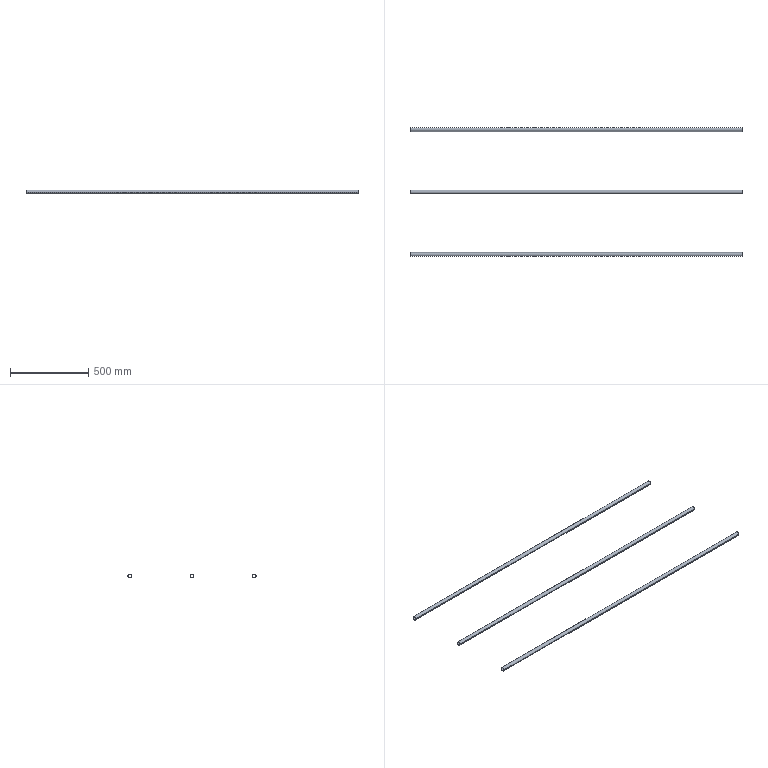Part | STEP file | Powder bin guardrail rail 5_Default<As Machined> | 3 solids | 18 faces | box 2128 x 825 x 25 mm | volume 706805 mm3 | cylinder 12 | plane 6 | commonest cylinder face diameters 22 x6 25 x6
STEP:
#1=CARTESIAN_POINT('',(0.,0.,0.));
#2=DIRECTION('',(0.,0.,1.));
#3=DIRECTION('',(1.,0.,0.));
#4=AXIS2_PLACEMENT_3D('',#1,#2,#3);
#5=CARTESIAN_POINT('',(1063.75,812.5,0.));
#6=VERTEX_POINT('',#5);
#7=CARTESIAN_POINT('',(1063.75,787.5,0.));
#8=VERTEX_POINT('',#7);
#9=CARTESIAN_POINT('',(1063.75,800.,0.));
#10=DIRECTION('',(1.,0.,0.));
#11=DIRECTION('',(0.,1.,0.));
#12=AXIS2_PLACEMENT_3D('',#9,#10,#11);
#13=CIRCLE('',#12,12.5);
#14=CARTESIAN_POINT('',(1063.75,800.,0.));
#15=DIRECTION('',(-1.,0.,0.));
#16=DIRECTION('',(0.,-1.,0.));
#17=AXIS2_PLACEMENT_3D('',#14,#15,#16);
#18=CYLINDRICAL_SURFACE('',#17,12.5);
#19=CARTESIAN_POINT('',(3.142,0.));
#20=DIRECTION('',(-1.,0.));
#21=VECTOR('',#20,1.);
#22=LINE('',#19,#21);
#23=(GEOMETRIC_REPRESENTATION_CONTEXT(2)PARAMETRIC_REPRESENTATION_CONTEXT()REPRESENTATION_CONTEXT('',''));
#24=DEFINITIONAL_REPRESENTATION('',(#22),#23);
#25=PCURVE('',#18,#24);
#26=CARTESIAN_POINT('',(1063.75,800.,0.));
#27=DIRECTION('',(1.,0.,0.));
#28=DIRECTION('',(0.,1.,0.));
#29=AXIS2_PLACEMENT_3D('',#26,#27,#28);
#30=PLANE('',#29);
#31=CARTESIAN_POINT('',(0.,0.));
#32=DIRECTION('',(1.,0.));
#33=AXIS2_PLACEMENT_2D('',#31,#32);
#34=CIRCLE('',#33,12.5);
#35=(GEOMETRIC_REPRESENTATION_CONTEXT(2)PARAMETRIC_REPRESENTATION_CONTEXT()REPRESENTATION_CONTEXT('',''));
#36=DEFINITIONAL_REPRESENTATION('',(#34),#35);
#37=PCURVE('',#30,#36);
#38=SURFACE_CURVE('',#13,(#25,#37),.PCURVE_S1.);
#39=EDGE_CURVE('',#6,#8,#38,.T.);
#40=ORIENTED_EDGE('',*,*,#39,.F.);
#41=CARTESIAN_POINT('',(-1063.75,812.5,0.));
#42=VERTEX_POINT('',#41);
#43=CARTESIAN_POINT('',(1063.75,812.5,0.));
#44=DIRECTION('',(-1.,0.,0.));
#45=VECTOR('',#44,1.);
#46=LINE('',#43,#45);
#47=CARTESIAN_POINT('',(3.142,0.));
#48=DIRECTION('',(0.,1.));
#49=VECTOR('',#48,1.);
#50=LINE('',#47,#49);
#51=(GEOMETRIC_REPRESENTATION_CONTEXT(2)PARAMETRIC_REPRESENTATION_CONTEXT()REPRESENTATION_CONTEXT('',''));
#52=DEFINITIONAL_REPRESENTATION('',(#50),#51);
#53=PCURVE('',#18,#52);
#54=CARTESIAN_POINT('',(1063.75,800.,0.));
#55=DIRECTION('',(-1.,0.,0.));
#56=DIRECTION('',(0.,-1.,0.));
#57=AXIS2_PLACEMENT_3D('',#54,#55,#56);
#58=CYLINDRICAL_SURFACE('',#57,12.5);
#59=CARTESIAN_POINT('',(3.142,0.));
#60=DIRECTION('',(0.,1.));
#61=VECTOR('',#60,1.);
#62=LINE('',#59,#61);
#63=(GEOMETRIC_REPRESENTATION_CONTEXT(2)PARAMETRIC_REPRESENTATION_CONTEXT()REPRESENTATION_CONTEXT('',''));
#64=DEFINITIONAL_REPRESENTATION('',(#62),#63);
#65=PCURVE('',#58,#64);
#66=SURFACE_CURVE('',#46,(#53,#65),.PCURVE_S1.);
#67=EDGE_CURVE('',#6,#42,#66,.T.);
#68=ORIENTED_EDGE('',*,*,#67,.T.);
#69=CARTESIAN_POINT('',(-1063.75,787.5,0.));
#70=VERTEX_POINT('',#69);
#71=CARTESIAN_POINT('',(-1063.75,800.,0.));
#72=DIRECTION('',(1.,0.,0.));
#73=DIRECTION('',(0.,1.,0.));
#74=AXIS2_PLACEMENT_3D('',#71,#72,#73);
#75=CIRCLE('',#74,12.5);
#76=CARTESIAN_POINT('',(3.142,2127.5));
#77=DIRECTION('',(-1.,0.));
#78=VECTOR('',#77,1.);
#79=LINE('',#76,#78);
#80=(GEOMETRIC_REPRESENTATION_CONTEXT(2)PARAMETRIC_REPRESENTATION_CONTEXT()REPRESENTATION_CONTEXT('',''));
#81=DEFINITIONAL_REPRESENTATION('',(#79),#80);
#82=PCURVE('',#18,#81);
#83=CARTESIAN_POINT('',(-1063.75,800.,0.));
#84=DIRECTION('',(1.,0.,0.));
#85=DIRECTION('',(0.,1.,0.));
#86=AXIS2_PLACEMENT_3D('',#83,#84,#85);
#87=PLANE('',#86);
#88=CARTESIAN_POINT('',(0.,0.));
#89=DIRECTION('',(1.,0.));
#90=AXIS2_PLACEMENT_2D('',#88,#89);
#91=CIRCLE('',#90,12.5);
#92=(GEOMETRIC_REPRESENTATION_CONTEXT(2)PARAMETRIC_REPRESENTATION_CONTEXT()REPRESENTATION_CONTEXT('',''));
#93=DEFINITIONAL_REPRESENTATION('',(#91),#92);
#94=PCURVE('',#87,#93);
#95=SURFACE_CURVE('',#75,(#82,#94),.PCURVE_S1.);
#96=EDGE_CURVE('',#42,#70,#95,.T.);
#97=ORIENTED_EDGE('',*,*,#96,.T.);
#98=CARTESIAN_POINT('',(1063.75,787.5,0.));
#99=DIRECTION('',(-1.,0.,0.));
#100=VECTOR('',#99,1.);
#101=LINE('',#98,#100);
#102=CARTESIAN_POINT('',(0.,0.));
#103=DIRECTION('',(0.,1.));
#104=VECTOR('',#103,1.);
#105=LINE('',#102,#104);
#106=(GEOMETRIC_REPRESENTATION_CONTEXT(2)PARAMETRIC_REPRESENTATION_CONTEXT()REPRESENTATION_CONTEXT('',''));
#107=DEFINITIONAL_REPRESENTATION('',(#105),#106);
#108=PCURVE('',#18,#107);
#109=CARTESIAN_POINT('',(6.283,0.));
#110=DIRECTION('',(0.,1.));
#111=VECTOR('',#110,1.);
#112=LINE('',#109,#111);
#113=(GEOMETRIC_REPRESENTATION_CONTEXT(2)PARAMETRIC_REPRESENTATION_CONTEXT()REPRESENTATION_CONTEXT('',''));
#114=DEFINITIONAL_REPRESENTATION('',(#112),#113);
#115=PCURVE('',#58,#114);
#116=SURFACE_CURVE('',#101,(#108,#115),.PCURVE_S1.);
#117=EDGE_CURVE('',#8,#70,#116,.T.);
#118=ORIENTED_EDGE('',*,*,#117,.F.);
#119=EDGE_LOOP('',(#40,#68,#97,#118));
#120=FACE_BOUND('',#119,.T.);
#121=ADVANCED_FACE('',(#120),#18,.T.);
#122=CARTESIAN_POINT('',(1063.75,789.,0.));
#123=VERTEX_POINT('',#122);
#124=CARTESIAN_POINT('',(-1063.75,789.,0.));
#125=VERTEX_POINT('',#124);
#126=CARTESIAN_POINT('',(1063.75,789.,0.));
#127=DIRECTION('',(-1.,0.,0.));
#128=VECTOR('',#127,1.);
#129=LINE('',#126,#128);
#130=CARTESIAN_POINT('',(1063.75,800.,0.));
#131=DIRECTION('',(-1.,0.,0.));
#132=DIRECTION('',(0.,-1.,0.));
#133=AXIS2_PLACEMENT_3D('',#130,#131,#132);
#134=CYLINDRICAL_SURFACE('',#133,11.);
#135=CARTESIAN_POINT('',(6.283,0.));
#136=DIRECTION('',(0.,1.));
#137=VECTOR('',#136,1.);
#138=LINE('',#135,#137);
#139=(GEOMETRIC_REPRESENTATION_CONTEXT(2)PARAMETRIC_REPRESENTATION_CONTEXT()REPRESENTATION_CONTEXT('',''));
#140=DEFINITIONAL_REPRESENTATION('',(#138),#139);
#141=PCURVE('',#134,#140);
#142=CARTESIAN_POINT('',(1063.75,800.,0.));
#143=DIRECTION('',(-1.,0.,0.));
#144=DIRECTION('',(0.,-1.,0.));
#145=AXIS2_PLACEMENT_3D('',#142,#143,#144);
#146=CYLINDRICAL_SURFACE('',#145,11.);
#147=CARTESIAN_POINT('',(0.,0.));
#148=DIRECTION('',(0.,1.));
#149=VECTOR('',#148,1.);
#150=LINE('',#147,#149);
#151=(GEOMETRIC_REPRESENTATION_CONTEXT(2)PARAMETRIC_REPRESENTATION_CONTEXT()REPRESENTATION_CONTEXT('',''));
#152=DEFINITIONAL_REPRESENTATION('',(#150),#151);
#153=PCURVE('',#146,#152);
#154=SURFACE_CURVE('',#129,(#141,#153),.PCURVE_S1.);
#155=EDGE_CURVE('',#123,#125,#154,.T.);
#156=ORIENTED_EDGE('',*,*,#155,.T.);
#157=CARTESIAN_POINT('',(-1063.75,811.,0.));
#158=VERTEX_POINT('',#157);
#159=CARTESIAN_POINT('',(-1063.75,800.,0.));
#160=DIRECTION('',(1.,0.,0.));
#161=DIRECTION('',(0.,1.,0.));
#162=AXIS2_PLACEMENT_3D('',#159,#160,#161);
#163=CIRCLE('',#162,11.);
#164=CARTESIAN_POINT('',(9.425,2127.5));
#165=DIRECTION('',(-1.,0.));
#166=VECTOR('',#165,1.);
#167=LINE('',#164,#166);
#168=(GEOMETRIC_REPRESENTATION_CONTEXT(2)PARAMETRIC_REPRESENTATION_CONTEXT()REPRESENTATION_CONTEXT('',''));
#169=DEFINITIONAL_REPRESENTATION('',(#167),#168);
#170=PCURVE('',#134,#169);
#171=CARTESIAN_POINT('',(0.,0.));
#172=DIRECTION('',(1.,0.));
#173=AXIS2_PLACEMENT_2D('',#171,#172);
#174=CIRCLE('',#173,11.);
#175=(GEOMETRIC_REPRESENTATION_CONTEXT(2)PARAMETRIC_REPRESENTATION_CONTEXT()REPRESENTATION_CONTEXT('',''));
#176=DEFINITIONAL_REPRESENTATION('',(#174),#175);
#177=PCURVE('',#87,#176);
#178=SURFACE_CURVE('',#163,(#170,#177),.PCURVE_S1.);
#179=EDGE_CURVE('',#125,#158,#178,.T.);
#180=ORIENTED_EDGE('',*,*,#179,.T.);
#181=CARTESIAN_POINT('',(1063.75,811.,0.));
#182=VERTEX_POINT('',#181);
#183=CARTESIAN_POINT('',(1063.75,811.,0.));
#184=DIRECTION('',(-1.,0.,0.));
#185=VECTOR('',#184,1.);
#186=LINE('',#183,#185);
#187=CARTESIAN_POINT('',(3.142,0.));
#188=DIRECTION('',(0.,1.));
#189=VECTOR('',#188,1.);
#190=LINE('',#187,#189);
#191=(GEOMETRIC_REPRESENTATION_CONTEXT(2)PARAMETRIC_REPRESENTATION_CONTEXT()REPRESENTATION_CONTEXT('',''));
#192=DEFINITIONAL_REPRESENTATION('',(#190),#191);
#193=PCURVE('',#134,#192);
#194=CARTESIAN_POINT('',(3.142,0.));
#195=DIRECTION('',(0.,1.));
#196=VECTOR('',#195,1.);
#197=LINE('',#194,#196);
#198=(GEOMETRIC_REPRESENTATION_CONTEXT(2)PARAMETRIC_REPRESENTATION_CONTEXT()REPRESENTATION_CONTEXT('',''));
#199=DEFINITIONAL_REPRESENTATION('',(#197),#198);
#200=PCURVE('',#146,#199);
#201=SURFACE_CURVE('',#186,(#193,#200),.PCURVE_S1.);
#202=EDGE_CURVE('',#182,#158,#201,.T.);
#203=ORIENTED_EDGE('',*,*,#202,.F.);
#204=CARTESIAN_POINT('',(1063.75,800.,0.));
#205=DIRECTION('',(1.,0.,0.));
#206=DIRECTION('',(0.,1.,0.));
#207=AXIS2_PLACEMENT_3D('',#204,#205,#206);
#208=CIRCLE('',#207,11.);
#209=CARTESIAN_POINT('',(9.425,0.));
#210=DIRECTION('',(-1.,0.));
#211=VECTOR('',#210,1.);
#212=LINE('',#209,#211);
#213=(GEOMETRIC_REPRESENTATION_CONTEXT(2)PARAMETRIC_REPRESENTATION_CONTEXT()REPRESENTATION_CONTEXT('',''));
#214=DEFINITIONAL_REPRESENTATION('',(#212),#213);
#215=PCURVE('',#134,#214);
#216=CARTESIAN_POINT('',(0.,0.));
#217=DIRECTION('',(1.,0.));
#218=AXIS2_PLACEMENT_2D('',#216,#217);
#219=CIRCLE('',#218,11.);
#220=(GEOMETRIC_REPRESENTATION_CONTEXT(2)PARAMETRIC_REPRESENTATION_CONTEXT()REPRESENTATION_CONTEXT('',''));
#221=DEFINITIONAL_REPRESENTATION('',(#219),#220);
#222=PCURVE('',#30,#221);
#223=SURFACE_CURVE('',#208,(#215,#222),.PCURVE_S1.);
#224=EDGE_CURVE('',#123,#182,#223,.T.);
#225=ORIENTED_EDGE('',*,*,#224,.F.);
#226=EDGE_LOOP('',(#156,#180,#203,#225));
#227=FACE_BOUND('',#226,.F.);
#228=ADVANCED_FACE('',(#227),#134,.F.);
#229=CARTESIAN_POINT('',(-1063.75,800.,0.));
#230=DIRECTION('',(1.,0.,0.));
#231=DIRECTION('',(0.,1.,0.));
#232=AXIS2_PLACEMENT_3D('',#229,#230,#231);
#233=CIRCLE('',#232,11.);
#234=CARTESIAN_POINT('',(3.142,2127.5));
#235=DIRECTION('',(-1.,0.));
#236=VECTOR('',#235,1.);
#237=LINE('',#234,#236);
#238=(GEOMETRIC_REPRESENTATION_CONTEXT(2)PARAMETRIC_REPRESENTATION_CONTEXT()REPRESENTATION_CONTEXT('',''));
#239=DEFINITIONAL_REPRESENTATION('',(#237),#238);
#240=PCURVE('',#146,#239);
#241=CARTESIAN_POINT('',(0.,0.));
#242=DIRECTION('',(1.,0.));
#243=AXIS2_PLACEMENT_2D('',#241,#242);
#244=CIRCLE('',#243,11.);
#245=(GEOMETRIC_REPRESENTATION_CONTEXT(2)PARAMETRIC_REPRESENTATION_CONTEXT()REPRESENTATION_CONTEXT('',''));
#246=DEFINITIONAL_REPRESENTATION('',(#244),#245);
#247=PCURVE('',#87,#246);
#248=SURFACE_CURVE('',#233,(#240,#247),.PCURVE_S1.);
#249=EDGE_CURVE('',#158,#125,#248,.T.);
#250=ORIENTED_EDGE('',*,*,#249,.T.);
#251=ORIENTED_EDGE('',*,*,#155,.F.);
#252=CARTESIAN_POINT('',(1063.75,800.,0.));
#253=DIRECTION('',(1.,0.,0.));
#254=DIRECTION('',(0.,1.,0.));
#255=AXIS2_PLACEMENT_3D('',#252,#253,#254);
#256=CIRCLE('',#255,11.);
#257=CARTESIAN_POINT('',(3.142,0.));
#258=DIRECTION('',(-1.,0.));
#259=VECTOR('',#258,1.);
#260=LINE('',#257,#259);
#261=(GEOMETRIC_REPRESENTATION_CONTEXT(2)PARAMETRIC_REPRESENTATION_CONTEXT()REPRESENTATION_CONTEXT('',''));
#262=DEFINITIONAL_REPRESENTATION('',(#260),#261);
#263=PCURVE('',#146,#262);
#264=CARTESIAN_POINT('',(0.,0.));
#265=DIRECTION('',(1.,0.));
#266=AXIS2_PLACEMENT_2D('',#264,#265);
#267=CIRCLE('',#266,11.);
#268=(GEOMETRIC_REPRESENTATION_CONTEXT(2)PARAMETRIC_REPRESENTATION_CONTEXT()REPRESENTATION_CONTEXT('',''));
#269=DEFINITIONAL_REPRESENTATION('',(#267),#268);
#270=PCURVE('',#30,#269);
#271=SURFACE_CURVE('',#256,(#263,#270),.PCURVE_S1.);
#272=EDGE_CURVE('',#182,#123,#271,.T.);
#273=ORIENTED_EDGE('',*,*,#272,.F.);
#274=ORIENTED_EDGE('',*,*,#202,.T.);
#275=EDGE_LOOP('',(#250,#251,#273,#274));
#276=FACE_BOUND('',#275,.F.);
#277=ADVANCED_FACE('',(#276),#146,.F.);
#278=ORIENTED_EDGE('',*,*,#67,.F.);
#279=CARTESIAN_POINT('',(1063.75,800.,0.));
#280=DIRECTION('',(1.,0.,0.));
#281=DIRECTION('',(0.,1.,0.));
#282=AXIS2_PLACEMENT_3D('',#279,#280,#281);
#283=CIRCLE('',#282,12.5);
#284=CARTESIAN_POINT('',(9.425,0.));
#285=DIRECTION('',(-1.,0.));
#286=VECTOR('',#285,1.);
#287=LINE('',#284,#286);
#288=(GEOMETRIC_REPRESENTATION_CONTEXT(2)PARAMETRIC_REPRESENTATION_CONTEXT()REPRESENTATION_CONTEXT('',''));
#289=DEFINITIONAL_REPRESENTATION('',(#287),#288);
#290=PCURVE('',#58,#289);
#291=CARTESIAN_POINT('',(0.,0.));
#292=DIRECTION('',(1.,0.));
#293=AXIS2_PLACEMENT_2D('',#291,#292);
#294=CIRCLE('',#293,12.5);
#295=(GEOMETRIC_REPRESENTATION_CONTEXT(2)PARAMETRIC_REPRESENTATION_CONTEXT()REPRESENTATION_CONTEXT('',''));
#296=DEFINITIONAL_REPRESENTATION('',(#294),#295);
#297=PCURVE('',#30,#296);
#298=SURFACE_CURVE('',#283,(#290,#297),.PCURVE_S1.);
#299=EDGE_CURVE('',#8,#6,#298,.T.);
#300=ORIENTED_EDGE('',*,*,#299,.F.);
#301=ORIENTED_EDGE('',*,*,#117,.T.);
#302=CARTESIAN_POINT('',(-1063.75,800.,0.));
#303=DIRECTION('',(1.,0.,0.));
#304=DIRECTION('',(0.,1.,0.));
#305=AXIS2_PLACEMENT_3D('',#302,#303,#304);
#306=CIRCLE('',#305,12.5);
#307=CARTESIAN_POINT('',(9.425,2127.5));
#308=DIRECTION('',(-1.,0.));
#309=VECTOR('',#308,1.);
#310=LINE('',#307,#309);
#311=(GEOMETRIC_REPRESENTATION_CONTEXT(2)PARAMETRIC_REPRESENTATION_CONTEXT()REPRESENTATION_CONTEXT('',''));
#312=DEFINITIONAL_REPRESENTATION('',(#310),#311);
#313=PCURVE('',#58,#312);
#314=CARTESIAN_POINT('',(0.,0.));
#315=DIRECTION('',(1.,0.));
#316=AXIS2_PLACEMENT_2D('',#314,#315);
#317=CIRCLE('',#316,12.5);
#318=(GEOMETRIC_REPRESENTATION_CONTEXT(2)PARAMETRIC_REPRESENTATION_CONTEXT()REPRESENTATION_CONTEXT('',''));
#319=DEFINITIONAL_REPRESENTATION('',(#317),#318);
#320=PCURVE('',#87,#319);
#321=SURFACE_CURVE('',#306,(#313,#320),.PCURVE_S1.);
#322=EDGE_CURVE('',#70,#42,#321,.T.);
#323=ORIENTED_EDGE('',*,*,#322,.T.);
#324=EDGE_LOOP('',(#278,#300,#301,#323));
#325=FACE_BOUND('',#324,.T.);
#326=ADVANCED_FACE('',(#325),#58,.T.);
#327=ORIENTED_EDGE('',*,*,#224,.F.);
#328=ORIENTED_EDGE('',*,*,#272,.F.);
#329=EDGE_LOOP('',(#327,#328));
#330=FACE_BOUND('',#329,.T.);
#331=ORIENTED_EDGE('',*,*,#299,.T.);
#332=ORIENTED_EDGE('',*,*,#39,.T.);
#333=EDGE_LOOP('',(#331,#332));
#334=FACE_BOUND('',#333,.T.);
#335=ADVANCED_FACE('',(#330,#334),#30,.T.);
#336=ORIENTED_EDGE('',*,*,#179,.T.);
#337=ORIENTED_EDGE('',*,*,#249,.T.);
#338=EDGE_LOOP('',(#336,#337));
#339=FACE_BOUND('',#338,.T.);
#340=ORIENTED_EDGE('',*,*,#322,.F.);
#341=ORIENTED_EDGE('',*,*,#96,.F.);
#342=EDGE_LOOP('',(#340,#341));
#343=FACE_BOUND('',#342,.T.);
#344=ADVANCED_FACE('',(#339,#343),#87,.F.);
#345=CLOSED_SHELL('',(#121,#228,#277,#326,#335,#344));
#346=MANIFOLD_SOLID_BREP('',#345);
#347=CARTESIAN_POINT('',(1063.75,12.5,0.));
#348=VERTEX_POINT('',#347);
#349=CARTESIAN_POINT('',(1063.75,-12.5,0.));
#350=VERTEX_POINT('',#349);
#351=CARTESIAN_POINT('',(1063.75,0.,0.));
#352=DIRECTION('',(1.,0.,0.));
#353=DIRECTION('',(0.,1.,0.));
#354=AXIS2_PLACEMENT_3D('',#351,#352,#353);
#355=CIRCLE('',#354,12.5);
#356=CARTESIAN_POINT('',(1063.75,0.,0.));
#357=DIRECTION('',(-1.,0.,0.));
#358=DIRECTION('',(0.,-1.,0.));
#359=AXIS2_PLACEMENT_3D('',#356,#357,#358);
#360=CYLINDRICAL_SURFACE('',#359,12.5);
#361=CARTESIAN_POINT('',(3.142,0.));
#362=DIRECTION('',(-1.,0.));
#363=VECTOR('',#362,1.);
#364=LINE('',#361,#363);
#365=(GEOMETRIC_REPRESENTATION_CONTEXT(2)PARAMETRIC_REPRESENTATION_CONTEXT()REPRESENTATION_CONTEXT('',''));
#366=DEFINITIONAL_REPRESENTATION('',(#364),#365);
#367=PCURVE('',#360,#366);
#368=CARTESIAN_POINT('',(1063.75,0.,0.));
#369=DIRECTION('',(1.,0.,0.));
#370=DIRECTION('',(0.,1.,0.));
#371=AXIS2_PLACEMENT_3D('',#368,#369,#370);
#372=PLANE('',#371);
#373=CARTESIAN_POINT('',(0.,0.));
#374=DIRECTION('',(1.,0.));
#375=AXIS2_PLACEMENT_2D('',#373,#374);
#376=CIRCLE('',#375,12.5);
#377=(GEOMETRIC_REPRESENTATION_CONTEXT(2)PARAMETRIC_REPRESENTATION_CONTEXT()REPRESENTATION_CONTEXT('',''));
#378=DEFINITIONAL_REPRESENTATION('',(#376),#377);
#379=PCURVE('',#372,#378);
#380=SURFACE_CURVE('',#355,(#367,#379),.PCURVE_S1.);
#381=EDGE_CURVE('',#348,#350,#380,.T.);
#382=ORIENTED_EDGE('',*,*,#381,.F.);
#383=CARTESIAN_POINT('',(-1063.75,12.5,0.));
#384=VERTEX_POINT('',#383);
#385=CARTESIAN_POINT('',(1063.75,12.5,0.));
#386=DIRECTION('',(-1.,0.,0.));
#387=VECTOR('',#386,1.);
#388=LINE('',#385,#387);
#389=CARTESIAN_POINT('',(3.142,0.));
#390=DIRECTION('',(0.,1.));
#391=VECTOR('',#390,1.);
#392=LINE('',#389,#391);
#393=(GEOMETRIC_REPRESENTATION_CONTEXT(2)PARAMETRIC_REPRESENTATION_CONTEXT()REPRESENTATION_CONTEXT('',''));
#394=DEFINITIONAL_REPRESENTATION('',(#392),#393);
#395=PCURVE('',#360,#394);
#396=CARTESIAN_POINT('',(1063.75,0.,0.));
#397=DIRECTION('',(-1.,0.,0.));
#398=DIRECTION('',(0.,-1.,0.));
#399=AXIS2_PLACEMENT_3D('',#396,#397,#398);
#400=CYLINDRICAL_SURFACE('',#399,12.5);
#401=CARTESIAN_POINT('',(3.142,0.));
#402=DIRECTION('',(0.,1.));
#403=VECTOR('',#402,1.);
#404=LINE('',#401,#403);
#405=(GEOMETRIC_REPRESENTATION_CONTEXT(2)PARAMETRIC_REPRESENTATION_CONTEXT()REPRESENTATION_CONTEXT('',''));
#406=DEFINITIONAL_REPRESENTATION('',(#404),#405);
#407=PCURVE('',#400,#406);
#408=SURFACE_CURVE('',#388,(#395,#407),.PCURVE_S1.);
#409=EDGE_CURVE('',#348,#384,#408,.T.);
#410=ORIENTED_EDGE('',*,*,#409,.T.);
#411=CARTESIAN_POINT('',(-1063.75,-12.5,0.));
#412=VERTEX_POINT('',#411);
#413=CARTESIAN_POINT('',(-1063.75,0.,0.));
#414=DIRECTION('',(1.,0.,0.));
#415=DIRECTION('',(0.,1.,0.));
#416=AXIS2_PLACEMENT_3D('',#413,#414,#415);
#417=CIRCLE('',#416,12.5);
#418=CARTESIAN_POINT('',(3.142,2127.5));
#419=DIRECTION('',(-1.,0.));
#420=VECTOR('',#419,1.);
#421=LINE('',#418,#420);
#422=(GEOMETRIC_REPRESENTATION_CONTEXT(2)PARAMETRIC_REPRESENTATION_CONTEXT()REPRESENTATION_CONTEXT('',''));
#423=DEFINITIONAL_REPRESENTATION('',(#421),#422);
#424=PCURVE('',#360,#423);
#425=CARTESIAN_POINT('',(-1063.75,0.,0.));
#426=DIRECTION('',(1.,0.,0.));
#427=DIRECTION('',(0.,1.,0.));
#428=AXIS2_PLACEMENT_3D('',#425,#426,#427);
#429=PLANE('',#428);
#430=CARTESIAN_POINT('',(0.,0.));
#431=DIRECTION('',(1.,0.));
#432=AXIS2_PLACEMENT_2D('',#430,#431);
#433=CIRCLE('',#432,12.5);
#434=(GEOMETRIC_REPRESENTATION_CONTEXT(2)PARAMETRIC_REPRESENTATION_CONTEXT()REPRESENTATION_CONTEXT('',''));
#435=DEFINITIONAL_REPRESENTATION('',(#433),#434);
#436=PCURVE('',#429,#435);
#437=SURFACE_CURVE('',#417,(#424,#436),.PCURVE_S1.);
#438=EDGE_CURVE('',#384,#412,#437,.T.);
#439=ORIENTED_EDGE('',*,*,#438,.T.);
#440=CARTESIAN_POINT('',(1063.75,-12.5,0.));
#441=DIRECTION('',(-1.,0.,0.));
#442=VECTOR('',#441,1.);
#443=LINE('',#440,#442);
#444=CARTESIAN_POINT('',(0.,0.));
#445=DIRECTION('',(0.,1.));
#446=VECTOR('',#445,1.);
#447=LINE('',#444,#446);
#448=(GEOMETRIC_REPRESENTATION_CONTEXT(2)PARAMETRIC_REPRESENTATION_CONTEXT()REPRESENTATION_CONTEXT('',''));
#449=DEFINITIONAL_REPRESENTATION('',(#447),#448);
#450=PCURVE('',#360,#449);
#451=CARTESIAN_POINT('',(6.283,0.));
#452=DIRECTION('',(0.,1.));
#453=VECTOR('',#452,1.);
#454=LINE('',#451,#453);
#455=(GEOMETRIC_REPRESENTATION_CONTEXT(2)PARAMETRIC_REPRESENTATION_CONTEXT()REPRESENTATION_CONTEXT('',''));
#456=DEFINITIONAL_REPRESENTATION('',(#454),#455);
#457=PCURVE('',#400,#456);
#458=SURFACE_CURVE('',#443,(#450,#457),.PCURVE_S1.);
#459=EDGE_CURVE('',#350,#412,#458,.T.);
#460=ORIENTED_EDGE('',*,*,#459,.F.);
#461=EDGE_LOOP('',(#382,#410,#439,#460));
#462=FACE_BOUND('',#461,.T.);
#463=ADVANCED_FACE('',(#462),#360,.T.);
#464=CARTESIAN_POINT('',(1063.75,-11.,0.));
#465=VERTEX_POINT('',#464);
#466=CARTESIAN_POINT('',(-1063.75,-11.,0.));
#467=VERTEX_POINT('',#466);
#468=CARTESIAN_POINT('',(1063.75,-11.,0.));
#469=DIRECTION('',(-1.,0.,0.));
#470=VECTOR('',#469,1.);
#471=LINE('',#468,#470);
#472=CARTESIAN_POINT('',(1063.75,0.,0.));
#473=DIRECTION('',(-1.,0.,0.));
#474=DIRECTION('',(0.,-1.,0.));
#475=AXIS2_PLACEMENT_3D('',#472,#473,#474);
#476=CYLINDRICAL_SURFACE('',#475,11.);
#477=CARTESIAN_POINT('',(6.283,0.));
#478=DIRECTION('',(0.,1.));
#479=VECTOR('',#478,1.);
#480=LINE('',#477,#479);
#481=(GEOMETRIC_REPRESENTATION_CONTEXT(2)PARAMETRIC_REPRESENTATION_CONTEXT()REPRESENTATION_CONTEXT('',''));
#482=DEFINITIONAL_REPRESENTATION('',(#480),#481);
#483=PCURVE('',#476,#482);
#484=CARTESIAN_POINT('',(1063.75,0.,0.));
#485=DIRECTION('',(-1.,0.,0.));
#486=DIRECTION('',(0.,-1.,0.));
#487=AXIS2_PLACEMENT_3D('',#484,#485,#486);
#488=CYLINDRICAL_SURFACE('',#487,11.);
#489=CARTESIAN_POINT('',(0.,0.));
#490=DIRECTION('',(0.,1.));
#491=VECTOR('',#490,1.);
#492=LINE('',#489,#491);
#493=(GEOMETRIC_REPRESENTATION_CONTEXT(2)PARAMETRIC_REPRESENTATION_CONTEXT()REPRESENTATION_CONTEXT('',''));
#494=DEFINITIONAL_REPRESENTATION('',(#492),#493);
#495=PCURVE('',#488,#494);
#496=SURFACE_CURVE('',#471,(#483,#495),.PCURVE_S1.);
#497=EDGE_CURVE('',#465,#467,#496,.T.);
#498=ORIENTED_EDGE('',*,*,#497,.T.);
#499=CARTESIAN_POINT('',(-1063.75,11.,0.));
#500=VERTEX_POINT('',#499);
#501=CARTESIAN_POINT('',(-1063.75,0.,0.));
#502=DIRECTION('',(1.,0.,0.));
#503=DIRECTION('',(0.,1.,0.));
#504=AXIS2_PLACEMENT_3D('',#501,#502,#503);
#505=CIRCLE('',#504,11.);
#506=CARTESIAN_POINT('',(9.425,2127.5));
#507=DIRECTION('',(-1.,0.));
#508=VECTOR('',#507,1.);
#509=LINE('',#506,#508);
#510=(GEOMETRIC_REPRESENTATION_CONTEXT(2)PARAMETRIC_REPRESENTATION_CONTEXT()REPRESENTATION_CONTEXT('',''));
#511=DEFINITIONAL_REPRESENTATION('',(#509),#510);
#512=PCURVE('',#476,#511);
#513=CARTESIAN_POINT('',(0.,0.));
#514=DIRECTION('',(1.,0.));
#515=AXIS2_PLACEMENT_2D('',#513,#514);
#516=CIRCLE('',#515,11.);
#517=(GEOMETRIC_REPRESENTATION_CONTEXT(2)PARAMETRIC_REPRESENTATION_CONTEXT()REPRESENTATION_CONTEXT('',''));
#518=DEFINITIONAL_REPRESENTATION('',(#516),#517);
#519=PCURVE('',#429,#518);
#520=SURFACE_CURVE('',#505,(#512,#519),.PCURVE_S1.);
#521=EDGE_CURVE('',#467,#500,#520,.T.);
#522=ORIENTED_EDGE('',*,*,#521,.T.);
#523=CARTESIAN_POINT('',(1063.75,11.,0.));
#524=VERTEX_POINT('',#523);
#525=CARTESIAN_POINT('',(1063.75,11.,0.));
#526=DIRECTION('',(-1.,0.,0.));
#527=VECTOR('',#526,1.);
#528=LINE('',#525,#527);
#529=CARTESIAN_POINT('',(3.142,0.));
#530=DIRECTION('',(0.,1.));
#531=VECTOR('',#530,1.);
#532=LINE('',#529,#531);
#533=(GEOMETRIC_REPRESENTATION_CONTEXT(2)PARAMETRIC_REPRESENTATION_CONTEXT()REPRESENTATION_CONTEXT('',''));
#534=DEFINITIONAL_REPRESENTATION('',(#532),#533);
#535=PCURVE('',#476,#534);
#536=CARTESIAN_POINT('',(3.142,0.));
#537=DIRECTION('',(0.,1.));
#538=VECTOR('',#537,1.);
#539=LINE('',#536,#538);
#540=(GEOMETRIC_REPRESENTATION_CONTEXT(2)PARAMETRIC_REPRESENTATION_CONTEXT()REPRESENTATION_CONTEXT('',''));
#541=DEFINITIONAL_REPRESENTATION('',(#539),#540);
#542=PCURVE('',#488,#541);
#543=SURFACE_CURVE('',#528,(#535,#542),.PCURVE_S1.);
#544=EDGE_CURVE('',#524,#500,#543,.T.);
#545=ORIENTED_EDGE('',*,*,#544,.F.);
#546=CARTESIAN_POINT('',(1063.75,0.,0.));
#547=DIRECTION('',(1.,0.,0.));
#548=DIRECTION('',(0.,1.,0.));
#549=AXIS2_PLACEMENT_3D('',#546,#547,#548);
#550=CIRCLE('',#549,11.);
#551=CARTESIAN_POINT('',(9.425,0.));
#552=DIRECTION('',(-1.,0.));
#553=VECTOR('',#552,1.);
#554=LINE('',#551,#553);
#555=(GEOMETRIC_REPRESENTATION_CONTEXT(2)PARAMETRIC_REPRESENTATION_CONTEXT()REPRESENTATION_CONTEXT('',''));
#556=DEFINITIONAL_REPRESENTATION('',(#554),#555);
#557=PCURVE('',#476,#556);
#558=CARTESIAN_POINT('',(0.,0.));
#559=DIRECTION('',(1.,0.));
#560=AXIS2_PLACEMENT_2D('',#558,#559);
#561=CIRCLE('',#560,11.);
#562=(GEOMETRIC_REPRESENTATION_CONTEXT(2)PARAMETRIC_REPRESENTATION_CONTEXT()REPRESENTATION_CONTEXT('',''));
#563=DEFINITIONAL_REPRESENTATION('',(#561),#562);
#564=PCURVE('',#372,#563);
#565=SURFACE_CURVE('',#550,(#557,#564),.PCURVE_S1.);
#566=EDGE_CURVE('',#465,#524,#565,.T.);
#567=ORIENTED_EDGE('',*,*,#566,.F.);
#568=EDGE_LOOP('',(#498,#522,#545,#567));
#569=FACE_BOUND('',#568,.F.);
#570=ADVANCED_FACE('',(#569),#476,.F.);
#571=CARTESIAN_POINT('',(-1063.75,0.,0.));
#572=DIRECTION('',(1.,0.,0.));
#573=DIRECTION('',(0.,1.,0.));
#574=AXIS2_PLACEMENT_3D('',#571,#572,#573);
#575=CIRCLE('',#574,11.);
#576=CARTESIAN_POINT('',(3.142,2127.5));
#577=DIRECTION('',(-1.,0.));
#578=VECTOR('',#577,1.);
#579=LINE('',#576,#578);
#580=(GEOMETRIC_REPRESENTATION_CONTEXT(2)PARAMETRIC_REPRESENTATION_CONTEXT()REPRESENTATION_CONTEXT('',''));
#581=DEFINITIONAL_REPRESENTATION('',(#579),#580);
#582=PCURVE('',#488,#581);
#583=CARTESIAN_POINT('',(0.,0.));
#584=DIRECTION('',(1.,0.));
#585=AXIS2_PLACEMENT_2D('',#583,#584);
#586=CIRCLE('',#585,11.);
#587=(GEOMETRIC_REPRESENTATION_CONTEXT(2)PARAMETRIC_REPRESENTATION_CONTEXT()REPRESENTATION_CONTEXT('',''));
#588=DEFINITIONAL_REPRESENTATION('',(#586),#587);
#589=PCURVE('',#429,#588);
#590=SURFACE_CURVE('',#575,(#582,#589),.PCURVE_S1.);
#591=EDGE_CURVE('',#500,#467,#590,.T.);
#592=ORIENTED_EDGE('',*,*,#591,.T.);
#593=ORIENTED_EDGE('',*,*,#497,.F.);
#594=CARTESIAN_POINT('',(1063.75,0.,0.));
#595=DIRECTION('',(1.,0.,0.));
#596=DIRECTION('',(0.,1.,0.));
#597=AXIS2_PLACEMENT_3D('',#594,#595,#596);
#598=CIRCLE('',#597,11.);
#599=CARTESIAN_POINT('',(3.142,0.));
#600=DIRECTION('',(-1.,0.));
#601=VECTOR('',#600,1.);
#602=LINE('',#599,#601);
#603=(GEOMETRIC_REPRESENTATION_CONTEXT(2)PARAMETRIC_REPRESENTATION_CONTEXT()REPRESENTATION_CONTEXT('',''));
#604=DEFINITIONAL_REPRESENTATION('',(#602),#603);
#605=PCURVE('',#488,#604);
#606=CARTESIAN_POINT('',(0.,0.));
#607=DIRECTION('',(1.,0.));
#608=AXIS2_PLACEMENT_2D('',#606,#607);
#609=CIRCLE('',#608,11.);
#610=(GEOMETRIC_REPRESENTATION_CONTEXT(2)PARAMETRIC_REPRESENTATION_CONTEXT()REPRESENTATION_CONTEXT('',''));
#611=DEFINITIONAL_REPRESENTATION('',(#609),#610);
#612=PCURVE('',#372,#611);
#613=SURFACE_CURVE('',#598,(#605,#612),.PCURVE_S1.);
#614=EDGE_CURVE('',#524,#465,#613,.T.);
#615=ORIENTED_EDGE('',*,*,#614,.F.);
#616=ORIENTED_EDGE('',*,*,#544,.T.);
#617=EDGE_LOOP('',(#592,#593,#615,#616));
#618=FACE_BOUND('',#617,.F.);
#619=ADVANCED_FACE('',(#618),#488,.F.);
#620=ORIENTED_EDGE('',*,*,#409,.F.);
#621=CARTESIAN_POINT('',(1063.75,0.,0.));
#622=DIRECTION('',(1.,0.,0.));
#623=DIRECTION('',(0.,1.,0.));
#624=AXIS2_PLACEMENT_3D('',#621,#622,#623);
#625=CIRCLE('',#624,12.5);
#626=CARTESIAN_POINT('',(9.425,0.));
#627=DIRECTION('',(-1.,0.));
#628=VECTOR('',#627,1.);
#629=LINE('',#626,#628);
#630=(GEOMETRIC_REPRESENTATION_CONTEXT(2)PARAMETRIC_REPRESENTATION_CONTEXT()REPRESENTATION_CONTEXT('',''));
#631=DEFINITIONAL_REPRESENTATION('',(#629),#630);
#632=PCURVE('',#400,#631);
#633=CARTESIAN_POINT('',(0.,0.));
#634=DIRECTION('',(1.,0.));
#635=AXIS2_PLACEMENT_2D('',#633,#634);
#636=CIRCLE('',#635,12.5);
#637=(GEOMETRIC_REPRESENTATION_CONTEXT(2)PARAMETRIC_REPRESENTATION_CONTEXT()REPRESENTATION_CONTEXT('',''));
#638=DEFINITIONAL_REPRESENTATION('',(#636),#637);
#639=PCURVE('',#372,#638);
#640=SURFACE_CURVE('',#625,(#632,#639),.PCURVE_S1.);
#641=EDGE_CURVE('',#350,#348,#640,.T.);
#642=ORIENTED_EDGE('',*,*,#641,.F.);
#643=ORIENTED_EDGE('',*,*,#459,.T.);
#644=CARTESIAN_POINT('',(-1063.75,0.,0.));
#645=DIRECTION('',(1.,0.,0.));
#646=DIRECTION('',(0.,1.,0.));
#647=AXIS2_PLACEMENT_3D('',#644,#645,#646);
#648=CIRCLE('',#647,12.5);
#649=CARTESIAN_POINT('',(9.425,2127.5));
#650=DIRECTION('',(-1.,0.));
#651=VECTOR('',#650,1.);
#652=LINE('',#649,#651);
#653=(GEOMETRIC_REPRESENTATION_CONTEXT(2)PARAMETRIC_REPRESENTATION_CONTEXT()REPRESENTATION_CONTEXT('',''));
#654=DEFINITIONAL_REPRESENTATION('',(#652),#653);
#655=PCURVE('',#400,#654);
#656=CARTESIAN_POINT('',(0.,0.));
#657=DIRECTION('',(1.,0.));
#658=AXIS2_PLACEMENT_2D('',#656,#657);
#659=CIRCLE('',#658,12.5);
#660=(GEOMETRIC_REPRESENTATION_CONTEXT(2)PARAMETRIC_REPRESENTATION_CONTEXT()REPRESENTATION_CONTEXT('',''));
#661=DEFINITIONAL_REPRESENTATION('',(#659),#660);
#662=PCURVE('',#429,#661);
#663=SURFACE_CURVE('',#648,(#655,#662),.PCURVE_S1.);
#664=EDGE_CURVE('',#412,#384,#663,.T.);
#665=ORIENTED_EDGE('',*,*,#664,.T.);
#666=EDGE_LOOP('',(#620,#642,#643,#665));
#667=FACE_BOUND('',#666,.T.);
#668=ADVANCED_FACE('',(#667),#400,.T.);
#669=ORIENTED_EDGE('',*,*,#566,.F.);
#670=ORIENTED_EDGE('',*,*,#614,.F.);
#671=EDGE_LOOP('',(#669,#670));
#672=FACE_BOUND('',#671,.T.);
#673=ORIENTED_EDGE('',*,*,#641,.T.);
#674=ORIENTED_EDGE('',*,*,#381,.T.);
#675=EDGE_LOOP('',(#673,#674));
#676=FACE_BOUND('',#675,.T.);
#677=ADVANCED_FACE('',(#672,#676),#372,.T.);
#678=ORIENTED_EDGE('',*,*,#521,.T.);
#679=ORIENTED_EDGE('',*,*,#591,.T.);
#680=EDGE_LOOP('',(#678,#679));
#681=FACE_BOUND('',#680,.T.);
#682=ORIENTED_EDGE('',*,*,#664,.F.);
#683=ORIENTED_EDGE('',*,*,#438,.F.);
#684=EDGE_LOOP('',(#682,#683));
#685=FACE_BOUND('',#684,.T.);
#686=ADVANCED_FACE('',(#681,#685),#429,.F.);
#687=CLOSED_SHELL('',(#463,#570,#619,#668,#677,#686));
#688=MANIFOLD_SOLID_BREP('',#687);
#689=CARTESIAN_POINT('',(1063.75,412.5,0.));
#690=VERTEX_POINT('',#689);
#691=CARTESIAN_POINT('',(1063.75,387.5,0.));
#692=VERTEX_POINT('',#691);
#693=CARTESIAN_POINT('',(1063.75,400.,0.));
#694=DIRECTION('',(1.,0.,0.));
#695=DIRECTION('',(0.,1.,0.));
#696=AXIS2_PLACEMENT_3D('',#693,#694,#695);
#697=CIRCLE('',#696,12.5);
#698=CARTESIAN_POINT('',(1063.75,400.,0.));
#699=DIRECTION('',(-1.,0.,0.));
#700=DIRECTION('',(0.,-1.,0.));
#701=AXIS2_PLACEMENT_3D('',#698,#699,#700);
#702=CYLINDRICAL_SURFACE('',#701,12.5);
#703=CARTESIAN_POINT('',(3.142,0.));
#704=DIRECTION('',(-1.,0.));
#705=VECTOR('',#704,1.);
#706=LINE('',#703,#705);
#707=(GEOMETRIC_REPRESENTATION_CONTEXT(2)PARAMETRIC_REPRESENTATION_CONTEXT()REPRESENTATION_CONTEXT('',''));
#708=DEFINITIONAL_REPRESENTATION('',(#706),#707);
#709=PCURVE('',#702,#708);
#710=CARTESIAN_POINT('',(1063.75,400.,0.));
#711=DIRECTION('',(1.,0.,0.));
#712=DIRECTION('',(0.,1.,0.));
#713=AXIS2_PLACEMENT_3D('',#710,#711,#712);
#714=PLANE('',#713);
#715=CARTESIAN_POINT('',(0.,0.));
#716=DIRECTION('',(1.,0.));
#717=AXIS2_PLACEMENT_2D('',#715,#716);
#718=CIRCLE('',#717,12.5);
#719=(GEOMETRIC_REPRESENTATION_CONTEXT(2)PARAMETRIC_REPRESENTATION_CONTEXT()REPRESENTATION_CONTEXT('',''));
#720=DEFINITIONAL_REPRESENTATION('',(#718),#719);
#721=PCURVE('',#714,#720);
#722=SURFACE_CURVE('',#697,(#709,#721),.PCURVE_S1.);
#723=EDGE_CURVE('',#690,#692,#722,.T.);
#724=ORIENTED_EDGE('',*,*,#723,.F.);
#725=CARTESIAN_POINT('',(-1063.75,412.5,0.));
#726=VERTEX_POINT('',#725);
#727=CARTESIAN_POINT('',(1063.75,412.5,0.));
#728=DIRECTION('',(-1.,0.,0.));
#729=VECTOR('',#728,1.);
#730=LINE('',#727,#729);
#731=CARTESIAN_POINT('',(3.142,0.));
#732=DIRECTION('',(0.,1.));
#733=VECTOR('',#732,1.);
#734=LINE('',#731,#733);
#735=(GEOMETRIC_REPRESENTATION_CONTEXT(2)PARAMETRIC_REPRESENTATION_CONTEXT()REPRESENTATION_CONTEXT('',''));
#736=DEFINITIONAL_REPRESENTATION('',(#734),#735);
#737=PCURVE('',#702,#736);
#738=CARTESIAN_POINT('',(1063.75,400.,0.));
#739=DIRECTION('',(-1.,0.,0.));
#740=DIRECTION('',(0.,-1.,0.));
#741=AXIS2_PLACEMENT_3D('',#738,#739,#740);
#742=CYLINDRICAL_SURFACE('',#741,12.5);
#743=CARTESIAN_POINT('',(3.142,0.));
#744=DIRECTION('',(0.,1.));
#745=VECTOR('',#744,1.);
#746=LINE('',#743,#745);
#747=(GEOMETRIC_REPRESENTATION_CONTEXT(2)PARAMETRIC_REPRESENTATION_CONTEXT()REPRESENTATION_CONTEXT('',''));
#748=DEFINITIONAL_REPRESENTATION('',(#746),#747);
#749=PCURVE('',#742,#748);
#750=SURFACE_CURVE('',#730,(#737,#749),.PCURVE_S1.);
#751=EDGE_CURVE('',#690,#726,#750,.T.);
#752=ORIENTED_EDGE('',*,*,#751,.T.);
#753=CARTESIAN_POINT('',(-1063.75,387.5,0.));
#754=VERTEX_POINT('',#753);
#755=CARTESIAN_POINT('',(-1063.75,400.,0.));
#756=DIRECTION('',(1.,0.,0.));
#757=DIRECTION('',(0.,1.,0.));
#758=AXIS2_PLACEMENT_3D('',#755,#756,#757);
#759=CIRCLE('',#758,12.5);
#760=CARTESIAN_POINT('',(3.142,2127.5));
#761=DIRECTION('',(-1.,0.));
#762=VECTOR('',#761,1.);
#763=LINE('',#760,#762);
#764=(GEOMETRIC_REPRESENTATION_CONTEXT(2)PARAMETRIC_REPRESENTATION_CONTEXT()REPRESENTATION_CONTEXT('',''));
#765=DEFINITIONAL_REPRESENTATION('',(#763),#764);
#766=PCURVE('',#702,#765);
#767=CARTESIAN_POINT('',(-1063.75,400.,0.));
#768=DIRECTION('',(1.,0.,0.));
#769=DIRECTION('',(0.,1.,0.));
#770=AXIS2_PLACEMENT_3D('',#767,#768,#769);
#771=PLANE('',#770);
#772=CARTESIAN_POINT('',(0.,0.));
#773=DIRECTION('',(1.,0.));
#774=AXIS2_PLACEMENT_2D('',#772,#773);
#775=CIRCLE('',#774,12.5);
#776=(GEOMETRIC_REPRESENTATION_CONTEXT(2)PARAMETRIC_REPRESENTATION_CONTEXT()REPRESENTATION_CONTEXT('',''));
#777=DEFINITIONAL_REPRESENTATION('',(#775),#776);
#778=PCURVE('',#771,#777);
#779=SURFACE_CURVE('',#759,(#766,#778),.PCURVE_S1.);
#780=EDGE_CURVE('',#726,#754,#779,.T.);
#781=ORIENTED_EDGE('',*,*,#780,.T.);
#782=CARTESIAN_POINT('',(1063.75,387.5,0.));
#783=DIRECTION('',(-1.,0.,0.));
#784=VECTOR('',#783,1.);
#785=LINE('',#782,#784);
#786=CARTESIAN_POINT('',(0.,0.));
#787=DIRECTION('',(0.,1.));
#788=VECTOR('',#787,1.);
#789=LINE('',#786,#788);
#790=(GEOMETRIC_REPRESENTATION_CONTEXT(2)PARAMETRIC_REPRESENTATION_CONTEXT()REPRESENTATION_CONTEXT('',''));
#791=DEFINITIONAL_REPRESENTATION('',(#789),#790);
#792=PCURVE('',#702,#791);
#793=CARTESIAN_POINT('',(6.283,0.));
#794=DIRECTION('',(0.,1.));
#795=VECTOR('',#794,1.);
#796=LINE('',#793,#795);
#797=(GEOMETRIC_REPRESENTATION_CONTEXT(2)PARAMETRIC_REPRESENTATION_CONTEXT()REPRESENTATION_CONTEXT('',''));
#798=DEFINITIONAL_REPRESENTATION('',(#796),#797);
#799=PCURVE('',#742,#798);
#800=SURFACE_CURVE('',#785,(#792,#799),.PCURVE_S1.);
#801=EDGE_CURVE('',#692,#754,#800,.T.);
#802=ORIENTED_EDGE('',*,*,#801,.F.);
#803=EDGE_LOOP('',(#724,#752,#781,#802));
#804=FACE_BOUND('',#803,.T.);
#805=ADVANCED_FACE('',(#804),#702,.T.);
#806=CARTESIAN_POINT('',(1063.75,389.,0.));
#807=VERTEX_POINT('',#806);
#808=CARTESIAN_POINT('',(-1063.75,389.,0.));
#809=VERTEX_POINT('',#808);
#810=CARTESIAN_POINT('',(1063.75,389.,0.));
#811=DIRECTION('',(-1.,0.,0.));
#812=VECTOR('',#811,1.);
#813=LINE('',#810,#812);
#814=CARTESIAN_POINT('',(1063.75,400.,0.));
#815=DIRECTION('',(-1.,0.,0.));
#816=DIRECTION('',(0.,-1.,0.));
#817=AXIS2_PLACEMENT_3D('',#814,#815,#816);
#818=CYLINDRICAL_SURFACE('',#817,11.);
#819=CARTESIAN_POINT('',(6.283,0.));
#820=DIRECTION('',(0.,1.));
#821=VECTOR('',#820,1.);
#822=LINE('',#819,#821);
#823=(GEOMETRIC_REPRESENTATION_CONTEXT(2)PARAMETRIC_REPRESENTATION_CONTEXT()REPRESENTATION_CONTEXT('',''));
#824=DEFINITIONAL_REPRESENTATION('',(#822),#823);
#825=PCURVE('',#818,#824);
#826=CARTESIAN_POINT('',(1063.75,400.,0.));
#827=DIRECTION('',(-1.,0.,0.));
#828=DIRECTION('',(0.,-1.,0.));
#829=AXIS2_PLACEMENT_3D('',#826,#827,#828);
#830=CYLINDRICAL_SURFACE('',#829,11.);
#831=CARTESIAN_POINT('',(0.,0.));
#832=DIRECTION('',(0.,1.));
#833=VECTOR('',#832,1.);
#834=LINE('',#831,#833);
#835=(GEOMETRIC_REPRESENTATION_CONTEXT(2)PARAMETRIC_REPRESENTATION_CONTEXT()REPRESENTATION_CONTEXT('',''));
#836=DEFINITIONAL_REPRESENTATION('',(#834),#835);
#837=PCURVE('',#830,#836);
#838=SURFACE_CURVE('',#813,(#825,#837),.PCURVE_S1.);
#839=EDGE_CURVE('',#807,#809,#838,.T.);
#840=ORIENTED_EDGE('',*,*,#839,.T.);
#841=CARTESIAN_POINT('',(-1063.75,411.,0.));
#842=VERTEX_POINT('',#841);
#843=CARTESIAN_POINT('',(-1063.75,400.,0.));
#844=DIRECTION('',(1.,0.,0.));
#845=DIRECTION('',(0.,1.,0.));
#846=AXIS2_PLACEMENT_3D('',#843,#844,#845);
#847=CIRCLE('',#846,11.);
#848=CARTESIAN_POINT('',(9.425,2127.5));
#849=DIRECTION('',(-1.,0.));
#850=VECTOR('',#849,1.);
#851=LINE('',#848,#850);
#852=(GEOMETRIC_REPRESENTATION_CONTEXT(2)PARAMETRIC_REPRESENTATION_CONTEXT()REPRESENTATION_CONTEXT('',''));
#853=DEFINITIONAL_REPRESENTATION('',(#851),#852);
#854=PCURVE('',#818,#853);
#855=CARTESIAN_POINT('',(0.,0.));
#856=DIRECTION('',(1.,0.));
#857=AXIS2_PLACEMENT_2D('',#855,#856);
#858=CIRCLE('',#857,11.);
#859=(GEOMETRIC_REPRESENTATION_CONTEXT(2)PARAMETRIC_REPRESENTATION_CONTEXT()REPRESENTATION_CONTEXT('',''));
#860=DEFINITIONAL_REPRESENTATION('',(#858),#859);
#861=PCURVE('',#771,#860);
#862=SURFACE_CURVE('',#847,(#854,#861),.PCURVE_S1.);
#863=EDGE_CURVE('',#809,#842,#862,.T.);
#864=ORIENTED_EDGE('',*,*,#863,.T.);
#865=CARTESIAN_POINT('',(1063.75,411.,0.));
#866=VERTEX_POINT('',#865);
#867=CARTESIAN_POINT('',(1063.75,411.,0.));
#868=DIRECTION('',(-1.,0.,0.));
#869=VECTOR('',#868,1.);
#870=LINE('',#867,#869);
#871=CARTESIAN_POINT('',(3.142,0.));
#872=DIRECTION('',(0.,1.));
#873=VECTOR('',#872,1.);
#874=LINE('',#871,#873);
#875=(GEOMETRIC_REPRESENTATION_CONTEXT(2)PARAMETRIC_REPRESENTATION_CONTEXT()REPRESENTATION_CONTEXT('',''));
#876=DEFINITIONAL_REPRESENTATION('',(#874),#875);
#877=PCURVE('',#818,#876);
#878=CARTESIAN_POINT('',(3.142,0.));
#879=DIRECTION('',(0.,1.));
#880=VECTOR('',#879,1.);
#881=LINE('',#878,#880);
#882=(GEOMETRIC_REPRESENTATION_CONTEXT(2)PARAMETRIC_REPRESENTATION_CONTEXT()REPRESENTATION_CONTEXT('',''));
#883=DEFINITIONAL_REPRESENTATION('',(#881),#882);
#884=PCURVE('',#830,#883);
#885=SURFACE_CURVE('',#870,(#877,#884),.PCURVE_S1.);
#886=EDGE_CURVE('',#866,#842,#885,.T.);
#887=ORIENTED_EDGE('',*,*,#886,.F.);
#888=CARTESIAN_POINT('',(1063.75,400.,0.));
#889=DIRECTION('',(1.,0.,0.));
#890=DIRECTION('',(0.,1.,0.));
#891=AXIS2_PLACEMENT_3D('',#888,#889,#890);
#892=CIRCLE('',#891,11.);
#893=CARTESIAN_POINT('',(9.425,0.));
#894=DIRECTION('',(-1.,0.));
#895=VECTOR('',#894,1.);
#896=LINE('',#893,#895);
#897=(GEOMETRIC_REPRESENTATION_CONTEXT(2)PARAMETRIC_REPRESENTATION_CONTEXT()REPRESENTATION_CONTEXT('',''));
#898=DEFINITIONAL_REPRESENTATION('',(#896),#897);
#899=PCURVE('',#818,#898);
#900=CARTESIAN_POINT('',(0.,0.));
#901=DIRECTION('',(1.,0.));
#902=AXIS2_PLACEMENT_2D('',#900,#901);
#903=CIRCLE('',#902,11.);
#904=(GEOMETRIC_REPRESENTATION_CONTEXT(2)PARAMETRIC_REPRESENTATION_CONTEXT()REPRESENTATION_CONTEXT('',''));
#905=DEFINITIONAL_REPRESENTATION('',(#903),#904);
#906=PCURVE('',#714,#905);
#907=SURFACE_CURVE('',#892,(#899,#906),.PCURVE_S1.);
#908=EDGE_CURVE('',#807,#866,#907,.T.);
#909=ORIENTED_EDGE('',*,*,#908,.F.);
#910=EDGE_LOOP('',(#840,#864,#887,#909));
#911=FACE_BOUND('',#910,.F.);
#912=ADVANCED_FACE('',(#911),#818,.F.);
#913=CARTESIAN_POINT('',(-1063.75,400.,0.));
#914=DIRECTION('',(1.,0.,0.));
#915=DIRECTION('',(0.,1.,0.));
#916=AXIS2_PLACEMENT_3D('',#913,#914,#915);
#917=CIRCLE('',#916,11.);
#918=CARTESIAN_POINT('',(3.142,2127.5));
#919=DIRECTION('',(-1.,0.));
#920=VECTOR('',#919,1.);
#921=LINE('',#918,#920);
#922=(GEOMETRIC_REPRESENTATION_CONTEXT(2)PARAMETRIC_REPRESENTATION_CONTEXT()REPRESENTATION_CONTEXT('',''));
#923=DEFINITIONAL_REPRESENTATION('',(#921),#922);
#924=PCURVE('',#830,#923);
#925=CARTESIAN_POINT('',(0.,0.));
#926=DIRECTION('',(1.,0.));
#927=AXIS2_PLACEMENT_2D('',#925,#926);
#928=CIRCLE('',#927,11.);
#929=(GEOMETRIC_REPRESENTATION_CONTEXT(2)PARAMETRIC_REPRESENTATION_CONTEXT()REPRESENTATION_CONTEXT('',''));
#930=DEFINITIONAL_REPRESENTATION('',(#928),#929);
#931=PCURVE('',#771,#930);
#932=SURFACE_CURVE('',#917,(#924,#931),.PCURVE_S1.);
#933=EDGE_CURVE('',#842,#809,#932,.T.);
#934=ORIENTED_EDGE('',*,*,#933,.T.);
#935=ORIENTED_EDGE('',*,*,#839,.F.);
#936=CARTESIAN_POINT('',(1063.75,400.,0.));
#937=DIRECTION('',(1.,0.,0.));
#938=DIRECTION('',(0.,1.,0.));
#939=AXIS2_PLACEMENT_3D('',#936,#937,#938);
#940=CIRCLE('',#939,11.);
#941=CARTESIAN_POINT('',(3.142,0.));
#942=DIRECTION('',(-1.,0.));
#943=VECTOR('',#942,1.);
#944=LINE('',#941,#943);
#945=(GEOMETRIC_REPRESENTATION_CONTEXT(2)PARAMETRIC_REPRESENTATION_CONTEXT()REPRESENTATION_CONTEXT('',''));
#946=DEFINITIONAL_REPRESENTATION('',(#944),#945);
#947=PCURVE('',#830,#946);
#948=CARTESIAN_POINT('',(0.,0.));
#949=DIRECTION('',(1.,0.));
#950=AXIS2_PLACEMENT_2D('',#948,#949);
#951=CIRCLE('',#950,11.);
#952=(GEOMETRIC_REPRESENTATION_CONTEXT(2)PARAMETRIC_REPRESENTATION_CONTEXT()REPRESENTATION_CONTEXT('',''));
#953=DEFINITIONAL_REPRESENTATION('',(#951),#952);
#954=PCURVE('',#714,#953);
#955=SURFACE_CURVE('',#940,(#947,#954),.PCURVE_S1.);
#956=EDGE_CURVE('',#866,#807,#955,.T.);
#957=ORIENTED_EDGE('',*,*,#956,.F.);
#958=ORIENTED_EDGE('',*,*,#886,.T.);
#959=EDGE_LOOP('',(#934,#935,#957,#958));
#960=FACE_BOUND('',#959,.F.);
#961=ADVANCED_FACE('',(#960),#830,.F.);
#962=ORIENTED_EDGE('',*,*,#751,.F.);
#963=CARTESIAN_POINT('',(1063.75,400.,0.));
#964=DIRECTION('',(1.,0.,0.));
#965=DIRECTION('',(0.,1.,0.));
#966=AXIS2_PLACEMENT_3D('',#963,#964,#965);
#967=CIRCLE('',#966,12.5);
#968=CARTESIAN_POINT('',(9.425,0.));
#969=DIRECTION('',(-1.,0.));
#970=VECTOR('',#969,1.);
#971=LINE('',#968,#970);
#972=(GEOMETRIC_REPRESENTATION_CONTEXT(2)PARAMETRIC_REPRESENTATION_CONTEXT()REPRESENTATION_CONTEXT('',''));
#973=DEFINITIONAL_REPRESENTATION('',(#971),#972);
#974=PCURVE('',#742,#973);
#975=CARTESIAN_POINT('',(0.,0.));
#976=DIRECTION('',(1.,0.));
#977=AXIS2_PLACEMENT_2D('',#975,#976);
#978=CIRCLE('',#977,12.5);
#979=(GEOMETRIC_REPRESENTATION_CONTEXT(2)PARAMETRIC_REPRESENTATION_CONTEXT()REPRESENTATION_CONTEXT('',''));
#980=DEFINITIONAL_REPRESENTATION('',(#978),#979);
#981=PCURVE('',#714,#980);
#982=SURFACE_CURVE('',#967,(#974,#981),.PCURVE_S1.);
#983=EDGE_CURVE('',#692,#690,#982,.T.);
#984=ORIENTED_EDGE('',*,*,#983,.F.);
#985=ORIENTED_EDGE('',*,*,#801,.T.);
#986=CARTESIAN_POINT('',(-1063.75,400.,0.));
#987=DIRECTION('',(1.,0.,0.));
#988=DIRECTION('',(0.,1.,0.));
#989=AXIS2_PLACEMENT_3D('',#986,#987,#988);
#990=CIRCLE('',#989,12.5);
#991=CARTESIAN_POINT('',(9.425,2127.5));
#992=DIRECTION('',(-1.,0.));
#993=VECTOR('',#992,1.);
#994=LINE('',#991,#993);
#995=(GEOMETRIC_REPRESENTATION_CONTEXT(2)PARAMETRIC_REPRESENTATION_CONTEXT()REPRESENTATION_CONTEXT('',''));
#996=DEFINITIONAL_REPRESENTATION('',(#994),#995);
#997=PCURVE('',#742,#996);
#998=CARTESIAN_POINT('',(0.,0.));
#999=DIRECTION('',(1.,0.));
#1000=AXIS2_PLACEMENT_2D('',#998,#999);
#1001=CIRCLE('',#1000,12.5);
#1002=(GEOMETRIC_REPRESENTATION_CONTEXT(2)PARAMETRIC_REPRESENTATION_CONTEXT()REPRESENTATION_CONTEXT('',''));
#1003=DEFINITIONAL_REPRESENTATION('',(#1001),#1002);
#1004=PCURVE('',#771,#1003);
#1005=SURFACE_CURVE('',#990,(#997,#1004),.PCURVE_S1.);
#1006=EDGE_CURVE('',#754,#726,#1005,.T.);
#1007=ORIENTED_EDGE('',*,*,#1006,.T.);
#1008=EDGE_LOOP('',(#962,#984,#985,#1007));
#1009=FACE_BOUND('',#1008,.T.);
#1010=ADVANCED_FACE('',(#1009),#742,.T.);
#1011=ORIENTED_EDGE('',*,*,#908,.F.);
#1012=ORIENTED_EDGE('',*,*,#956,.F.);
#1013=EDGE_LOOP('',(#1011,#1012));
#1014=FACE_BOUND('',#1013,.T.);
#1015=ORIENTED_EDGE('',*,*,#983,.T.);
#1016=ORIENTED_EDGE('',*,*,#723,.T.);
#1017=EDGE_LOOP('',(#1015,#1016));
#1018=FACE_BOUND('',#1017,.T.);
#1019=ADVANCED_FACE('',(#1014,#1018),#714,.T.);
#1020=ORIENTED_EDGE('',*,*,#863,.T.);
#1021=ORIENTED_EDGE('',*,*,#933,.T.);
#1022=EDGE_LOOP('',(#1020,#1021));
#1023=FACE_BOUND('',#1022,.T.);
#1024=ORIENTED_EDGE('',*,*,#1006,.F.);
#1025=ORIENTED_EDGE('',*,*,#780,.F.);
#1026=EDGE_LOOP('',(#1024,#1025));
#1027=FACE_BOUND('',#1026,.T.);
#1028=ADVANCED_FACE('',(#1023,#1027),#771,.F.);
#1029=CLOSED_SHELL('',(#805,#912,#961,#1010,#1019,#1028));
#1030=MANIFOLD_SOLID_BREP('',#1029);
#1031=(LENGTH_UNIT()NAMED_UNIT(*)SI_UNIT(.MILLI.,.METRE.));
#1032=UNCERTAINTY_MEASURE_WITH_UNIT(LENGTH_MEASURE(0.0000001),#1031,'','');
#1033=(NAMED_UNIT(*)PLANE_ANGLE_UNIT()SI_UNIT($,.RADIAN.));
#1034=(NAMED_UNIT(*)SI_UNIT($,.STERADIAN.)SOLID_ANGLE_UNIT());
#1035=(GEOMETRIC_REPRESENTATION_CONTEXT(3)GLOBAL_UNCERTAINTY_ASSIGNED_CONTEXT((#1032))GLOBAL_UNIT_ASSIGNED_CONTEXT((#1031,#1033,#1034))REPRESENTATION_CONTEXT('',''));
#1036=SHAPE_REPRESENTATION('',(#4,#346,#688,#1030),#1035);